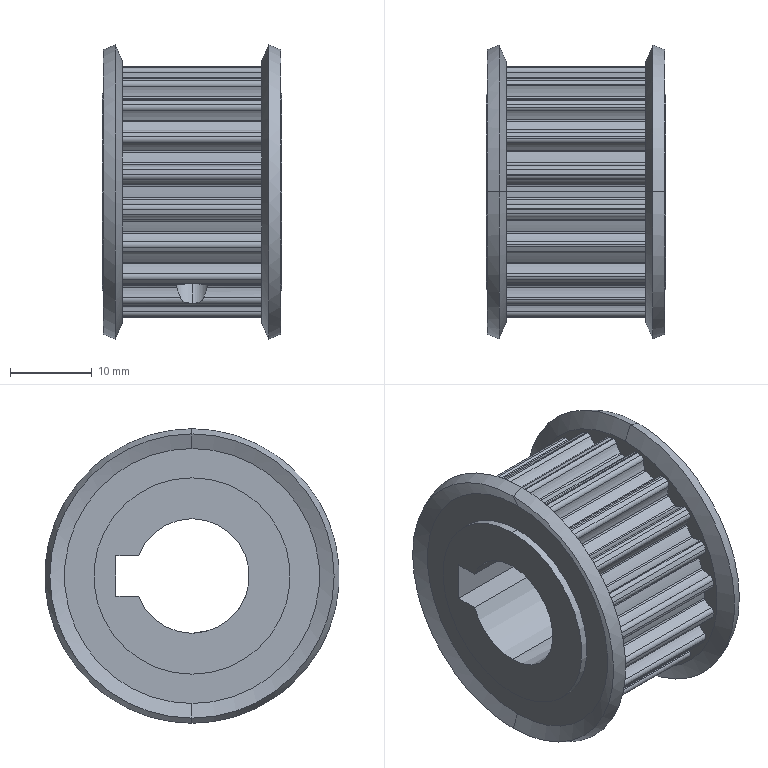Part | STEP file | 11-HTPA20S5M150_A_N14_a11 | 1 solid | 224 faces | box 22 x 36 x 36 mm | volume 11310 mm3 | cylinder 203 | cone 12 | plane 9 | commonest cylinder face diameters 0.5 x51 1.1 x50 6.55 x48 27.33 x23 30.87 x20 4.134 x4